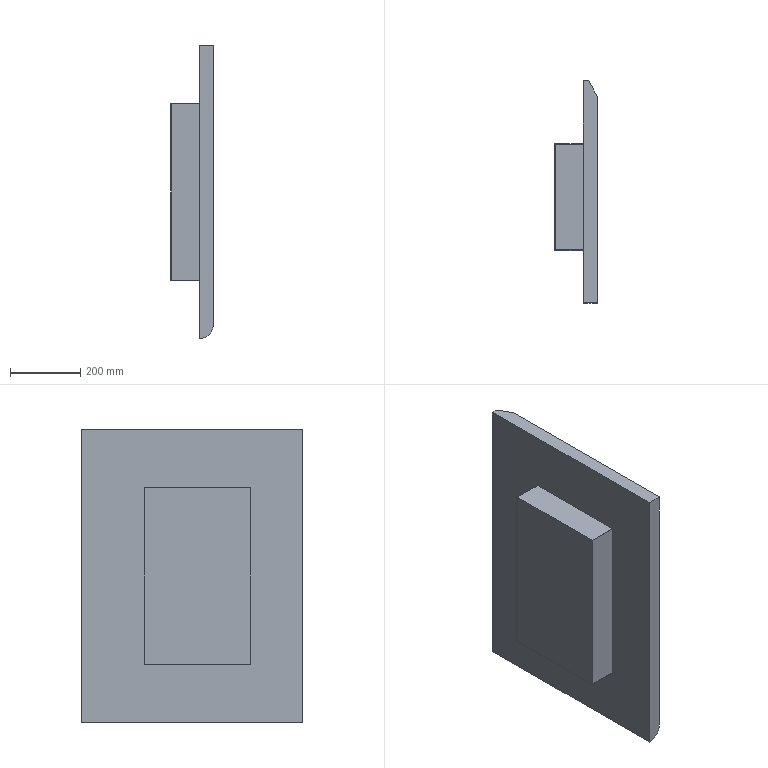Part | SolidWorks | features ICE 2, BossThin 1, CutThin 1, Extrusion 1, Fillet 1 | 1 solid | 27 faces | box 121.2 x 630 x 832.5 mm | volume 14657432 mm3 | plane 26 | cylinder 1 | commonest cylinder face diameters 80 x1
STEP:
#1=CARTESIAN_POINT('',(15.,0.,832.5));
#2=VERTEX_POINT('',#1);
#3=CARTESIAN_POINT('',(15.,0.,2.919));
#4=VERTEX_POINT('',#3);
#5=CARTESIAN_POINT('',(15.,0.,832.5));
#6=DIRECTION('',(0.,0.,-1.));
#7=VECTOR('',#6,1000.);
#8=LINE('',#5,#7);
#9=EDGE_CURVE('',#2,#4,#8,.T.);
#10=ORIENTED_EDGE('',*,*,#9,.T.);
#11=CARTESIAN_POINT('',(0.,0.,0.));
#12=VERTEX_POINT('',#11);
#13=CARTESIAN_POINT('',(0.,0.,40.));
#14=DIRECTION('',(0.,1.,0.));
#15=DIRECTION('',(0.,0.,-1.));
#16=AXIS2_PLACEMENT_3D('',#13,#14,#15);
#17=CIRCLE('',#16,40.);
#18=EDGE_CURVE('',#4,#12,#17,.T.);
#19=ORIENTED_EDGE('',*,*,#18,.T.);
#20=CARTESIAN_POINT('',(0.,0.,832.5));
#21=VERTEX_POINT('',#20);
#22=CARTESIAN_POINT('',(0.,0.,832.5));
#23=DIRECTION('',(0.,0.,-1.));
#24=VECTOR('',#23,1000.);
#25=LINE('',#22,#24);
#26=EDGE_CURVE('',#21,#12,#25,.T.);
#27=ORIENTED_EDGE('',*,*,#26,.F.);
#28=CARTESIAN_POINT('',(0.,0.,832.5));
#29=DIRECTION('',(-1.,0.,0.));
#30=VECTOR('',#29,1000.);
#31=LINE('',#28,#30);
#32=EDGE_CURVE('',#2,#21,#31,.T.);
#33=ORIENTED_EDGE('',*,*,#32,.F.);
#34=EDGE_LOOP('',(#10,#19,#27,#33));
#35=FACE_OUTER_BOUND('',#34,.T.);
#36=CARTESIAN_POINT('',(0.,0.,832.5));
#37=DIRECTION('',(0.,-1.,0.));
#38=DIRECTION('',(0.,0.,-1.));
#39=AXIS2_PLACEMENT_3D('',#36,#37,#38);
#40=PLANE('',#39);
#41=ADVANCED_FACE('',(#35),#40,.F.);
#42=CARTESIAN_POINT('',(0.,-178.8,165.05));
#43=VERTEX_POINT('',#42);
#44=CARTESIAN_POINT('',(0.,-178.8,667.45));
#45=VERTEX_POINT('',#44);
#46=CARTESIAN_POINT('',(0.,-178.8,832.5));
#47=DIRECTION('',(0.,0.,1.));
#48=VECTOR('',#47,1000.);
#49=LINE('',#46,#48);
#50=EDGE_CURVE('',#43,#45,#49,.T.);
#51=ORIENTED_EDGE('',*,*,#50,.T.);
#52=CARTESIAN_POINT('',(0.,-481.2,667.45));
#53=VERTEX_POINT('',#52);
#54=CARTESIAN_POINT('',(0.,0.,667.45));
#55=DIRECTION('',(0.,-1.,0.));
#56=VECTOR('',#55,1000.);
#57=LINE('',#54,#56);
#58=EDGE_CURVE('',#45,#53,#57,.T.);
#59=ORIENTED_EDGE('',*,*,#58,.T.);
#60=CARTESIAN_POINT('',(0.,-481.2,165.05));
#61=VERTEX_POINT('',#60);
#62=CARTESIAN_POINT('',(0.,-481.2,832.5));
#63=DIRECTION('',(0.,0.,-1.));
#64=VECTOR('',#63,1000.);
#65=LINE('',#62,#64);
#66=EDGE_CURVE('',#53,#61,#65,.T.);
#67=ORIENTED_EDGE('',*,*,#66,.T.);
#68=CARTESIAN_POINT('',(0.,0.,165.05));
#69=DIRECTION('',(0.,1.,0.));
#70=VECTOR('',#69,1000.);
#71=LINE('',#68,#70);
#72=EDGE_CURVE('',#61,#43,#71,.T.);
#73=ORIENTED_EDGE('',*,*,#72,.T.);
#74=EDGE_LOOP('',(#51,#59,#67,#73));
#75=FACE_BOUND('',#74,.T.);
#76=CARTESIAN_POINT('',(0.,-630.,0.));
#77=VERTEX_POINT('',#76);
#78=CARTESIAN_POINT('',(0.,0.,0.));
#79=DIRECTION('',(0.,-1.,0.));
#80=VECTOR('',#79,1000.);
#81=LINE('',#78,#80);
#82=EDGE_CURVE('',#12,#77,#81,.T.);
#83=ORIENTED_EDGE('',*,*,#82,.T.);
#84=CARTESIAN_POINT('',(0.,-630.,832.5));
#85=VERTEX_POINT('',#84);
#86=CARTESIAN_POINT('',(0.,-630.,832.5));
#87=DIRECTION('',(0.,0.,-1.));
#88=VECTOR('',#87,1000.);
#89=LINE('',#86,#88);
#90=EDGE_CURVE('',#85,#77,#89,.T.);
#91=ORIENTED_EDGE('',*,*,#90,.F.);
#92=CARTESIAN_POINT('',(0.,0.,832.5));
#93=DIRECTION('',(0.,-1.,0.));
#94=VECTOR('',#93,1000.);
#95=LINE('',#92,#94);
#96=EDGE_CURVE('',#21,#85,#95,.T.);
#97=ORIENTED_EDGE('',*,*,#96,.F.);
#98=ORIENTED_EDGE('',*,*,#26,.T.);
#99=EDGE_LOOP('',(#83,#91,#97,#98));
#100=FACE_OUTER_BOUND('',#99,.T.);
#101=CARTESIAN_POINT('',(0.,0.,832.5));
#102=DIRECTION('',(1.,0.,0.));
#103=DIRECTION('',(0.,1.,0.));
#104=AXIS2_PLACEMENT_3D('',#101,#102,#103);
#105=PLANE('',#104);
#106=ADVANCED_FACE('',(#75,#100),#105,.F.);
#107=ORIENTED_EDGE('',*,*,#90,.T.);
#108=CARTESIAN_POINT('',(40.,-630.,40.));
#109=VERTEX_POINT('',#108);
#110=CARTESIAN_POINT('',(0.,-630.,40.));
#111=DIRECTION('',(0.,-1.,0.));
#112=DIRECTION('',(0.,0.,1.));
#113=AXIS2_PLACEMENT_3D('',#110,#111,#112);
#114=CIRCLE('',#113,40.);
#115=EDGE_CURVE('',#77,#109,#114,.T.);
#116=ORIENTED_EDGE('',*,*,#115,.T.);
#117=CARTESIAN_POINT('',(40.,-630.,832.5));
#118=VERTEX_POINT('',#117);
#119=CARTESIAN_POINT('',(40.,-630.,832.5));
#120=DIRECTION('',(0.,0.,-1.));
#121=VECTOR('',#120,1000.);
#122=LINE('',#119,#121);
#123=EDGE_CURVE('',#118,#109,#122,.T.);
#124=ORIENTED_EDGE('',*,*,#123,.F.);
#125=CARTESIAN_POINT('',(0.,-630.,832.5));
#126=DIRECTION('',(1.,0.,0.));
#127=VECTOR('',#126,1000.);
#128=LINE('',#125,#127);
#129=EDGE_CURVE('',#85,#118,#128,.T.);
#130=ORIENTED_EDGE('',*,*,#129,.F.);
#131=EDGE_LOOP('',(#107,#116,#124,#130));
#132=FACE_OUTER_BOUND('',#131,.T.);
#133=CARTESIAN_POINT('',(0.,-630.,832.5));
#134=DIRECTION('',(0.,1.,0.));
#135=DIRECTION('',(0.,0.,1.));
#136=AXIS2_PLACEMENT_3D('',#133,#134,#135);
#137=PLANE('',#136);
#138=ADVANCED_FACE('',(#132),#137,.F.);
#139=CARTESIAN_POINT('',(40.,-144.501,465.45));
#140=VERTEX_POINT('',#139);
#141=CARTESIAN_POINT('',(40.,-144.501,367.05));
#142=VERTEX_POINT('',#141);
#143=CARTESIAN_POINT('',(40.,-144.501,464.25));
#144=DIRECTION('',(0.,0.,-1.));
#145=VECTOR('',#144,1000.);
#146=LINE('',#143,#145);
#147=EDGE_CURVE('',#140,#142,#146,.T.);
#148=ORIENTED_EDGE('',*,*,#147,.F.);
#149=CARTESIAN_POINT('',(40.,-102.101,465.45));
#150=VERTEX_POINT('',#149);
#151=CARTESIAN_POINT('',(40.,-103.301,465.45));
#152=DIRECTION('',(0.,-1.,0.));
#153=VECTOR('',#152,1000.);
#154=LINE('',#151,#153);
#155=EDGE_CURVE('',#150,#140,#154,.T.);
#156=ORIENTED_EDGE('',*,*,#155,.F.);
#157=CARTESIAN_POINT('',(40.,-102.101,367.05));
#158=VERTEX_POINT('',#157);
#159=CARTESIAN_POINT('',(40.,-102.101,464.25));
#160=DIRECTION('',(0.,0.,1.));
#161=VECTOR('',#160,1000.);
#162=LINE('',#159,#161);
#163=EDGE_CURVE('',#158,#150,#162,.T.);
#164=ORIENTED_EDGE('',*,*,#163,.F.);
#165=CARTESIAN_POINT('',(40.,-103.301,367.05));
#166=DIRECTION('',(0.,1.,0.));
#167=VECTOR('',#166,1000.);
#168=LINE('',#165,#167);
#169=EDGE_CURVE('',#142,#158,#168,.T.);
#170=ORIENTED_EDGE('',*,*,#169,.F.);
#171=EDGE_LOOP('',(#148,#156,#164,#170));
#172=FACE_BOUND('',#171,.T.);
#173=ORIENTED_EDGE('',*,*,#123,.T.);
#174=CARTESIAN_POINT('',(40.,-43.301,40.));
#175=VERTEX_POINT('',#174);
#176=CARTESIAN_POINT('',(40.,-630.,40.));
#177=DIRECTION('',(0.,1.,0.));
#178=VECTOR('',#177,1000.);
#179=LINE('',#176,#178);
#180=EDGE_CURVE('',#109,#175,#179,.T.);
#181=ORIENTED_EDGE('',*,*,#180,.T.);
#182=CARTESIAN_POINT('',(40.,-43.301,832.5));
#183=VERTEX_POINT('',#182);
#184=CARTESIAN_POINT('',(40.,-43.301,832.5));
#185=DIRECTION('',(0.,0.,-1.));
#186=VECTOR('',#185,1000.);
#187=LINE('',#184,#186);
#188=EDGE_CURVE('',#183,#175,#187,.T.);
#189=ORIENTED_EDGE('',*,*,#188,.F.);
#190=CARTESIAN_POINT('',(40.,-630.,832.5));
#191=DIRECTION('',(0.,1.,0.));
#192=VECTOR('',#191,1000.);
#193=LINE('',#190,#192);
#194=EDGE_CURVE('',#118,#183,#193,.T.);
#195=ORIENTED_EDGE('',*,*,#194,.F.);
#196=EDGE_LOOP('',(#173,#181,#189,#195));
#197=FACE_OUTER_BOUND('',#196,.T.);
#198=CARTESIAN_POINT('',(40.,-480.,666.25));
#199=VERTEX_POINT('',#198);
#200=CARTESIAN_POINT('',(40.,-480.,166.25));
#201=VERTEX_POINT('',#200);
#202=CARTESIAN_POINT('',(40.,-480.,666.25));
#203=DIRECTION('',(0.,0.,-1.));
#204=VECTOR('',#203,1000.);
#205=LINE('',#202,#204);
#206=EDGE_CURVE('',#199,#201,#205,.T.);
#207=ORIENTED_EDGE('',*,*,#206,.F.);
#208=CARTESIAN_POINT('',(40.,-180.,666.25));
#209=VERTEX_POINT('',#208);
#210=CARTESIAN_POINT('',(40.,-180.,666.25));
#211=DIRECTION('',(0.,-1.,0.));
#212=VECTOR('',#211,1000.);
#213=LINE('',#210,#212);
#214=EDGE_CURVE('',#209,#199,#213,.T.);
#215=ORIENTED_EDGE('',*,*,#214,.F.);
#216=CARTESIAN_POINT('',(40.,-180.,166.25));
#217=VERTEX_POINT('',#216);
#218=CARTESIAN_POINT('',(40.,-180.,666.25));
#219=DIRECTION('',(0.,0.,1.));
#220=VECTOR('',#219,1000.);
#221=LINE('',#218,#220);
#222=EDGE_CURVE('',#217,#209,#221,.T.);
#223=ORIENTED_EDGE('',*,*,#222,.F.);
#224=CARTESIAN_POINT('',(40.,-180.,166.25));
#225=DIRECTION('',(0.,1.,0.));
#226=VECTOR('',#225,1000.);
#227=LINE('',#224,#226);
#228=EDGE_CURVE('',#201,#217,#227,.T.);
#229=ORIENTED_EDGE('',*,*,#228,.F.);
#230=EDGE_LOOP('',(#207,#215,#223,#229));
#231=FACE_BOUND('',#230,.T.);
#232=CARTESIAN_POINT('',(40.,-630.,832.5));
#233=DIRECTION('',(-1.,0.,0.));
#234=DIRECTION('',(0.,-1.,0.));
#235=AXIS2_PLACEMENT_3D('',#232,#233,#234);
#236=PLANE('',#235);
#237=ADVANCED_FACE('',(#172,#197,#231),#236,.F.);
#238=ORIENTED_EDGE('',*,*,#188,.T.);
#239=CARTESIAN_POINT('',(40.,-43.301,40.));
#240=CARTESIAN_POINT('',(40.,-43.301,23.177));
#241=CARTESIAN_POINT('',(30.596,-27.012,9.228));
#242=CARTESIAN_POINT('',(15.,0.,2.919));
#243=(BOUNDED_CURVE()B_SPLINE_CURVE(3,(#239,#240,#241,#242),.UNSPECIFIED.,.F.,.F.)B_SPLINE_CURVE_WITH_KNOTS((4,4),(3.142,4.328),.UNSPECIFIED.)CURVE()GEOMETRIC_REPRESENTATION_ITEM()RATIONAL_B_SPLINE_CURVE((1.,0.8861,0.8861,1.))REPRESENTATION_ITEM(''));
#244=EDGE_CURVE('',#175,#4,#243,.T.);
#245=ORIENTED_EDGE('',*,*,#244,.T.);
#246=ORIENTED_EDGE('',*,*,#9,.F.);
#247=CARTESIAN_POINT('',(15.,0.,832.5));
#248=DIRECTION('',(-0.5,0.866,0.));
#249=VECTOR('',#248,1000.);
#250=LINE('',#247,#249);
#251=EDGE_CURVE('',#183,#2,#250,.T.);
#252=ORIENTED_EDGE('',*,*,#251,.F.);
#253=EDGE_LOOP('',(#238,#245,#246,#252));
#254=FACE_OUTER_BOUND('',#253,.T.);
#255=CARTESIAN_POINT('',(15.,0.,832.5));
#256=DIRECTION('',(-0.866,-0.5,0.));
#257=DIRECTION('',(0.5,-0.866,0.));
#258=AXIS2_PLACEMENT_3D('',#255,#256,#257);
#259=PLANE('',#258);
#260=ADVANCED_FACE('',(#254),#259,.F.);
#261=ORIENTED_EDGE('',*,*,#32,.T.);
#262=ORIENTED_EDGE('',*,*,#96,.T.);
#263=ORIENTED_EDGE('',*,*,#129,.T.);
#264=ORIENTED_EDGE('',*,*,#194,.T.);
#265=ORIENTED_EDGE('',*,*,#251,.T.);
#266=EDGE_LOOP('',(#261,#262,#263,#264,#265));
#267=FACE_OUTER_BOUND('',#266,.T.);
#268=CARTESIAN_POINT('',(0.,0.,832.5));
#269=DIRECTION('',(0.,0.,1.));
#270=DIRECTION('',(1.,0.,0.));
#271=AXIS2_PLACEMENT_3D('',#268,#269,#270);
#272=PLANE('',#271);
#273=ADVANCED_FACE('',(#267),#272,.T.);
#274=ORIENTED_EDGE('',*,*,#155,.T.);
#275=CARTESIAN_POINT('',(38.,-144.501,465.45));
#276=VERTEX_POINT('',#275);
#277=CARTESIAN_POINT('',(38.,-144.501,465.45));
#278=DIRECTION('',(1.,0.,0.));
#279=VECTOR('',#278,1000.);
#280=LINE('',#277,#279);
#281=EDGE_CURVE('',#276,#140,#280,.T.);
#282=ORIENTED_EDGE('',*,*,#281,.F.);
#283=CARTESIAN_POINT('',(38.,-102.101,465.45));
#284=VERTEX_POINT('',#283);
#285=CARTESIAN_POINT('',(38.,-103.301,465.45));
#286=DIRECTION('',(0.,-1.,0.));
#287=VECTOR('',#286,1000.);
#288=LINE('',#285,#287);
#289=EDGE_CURVE('',#284,#276,#288,.T.);
#290=ORIENTED_EDGE('',*,*,#289,.F.);
#291=CARTESIAN_POINT('',(38.,-102.101,465.45));
#292=DIRECTION('',(1.,0.,0.));
#293=VECTOR('',#292,1000.);
#294=LINE('',#291,#293);
#295=EDGE_CURVE('',#284,#150,#294,.T.);
#296=ORIENTED_EDGE('',*,*,#295,.T.);
#297=EDGE_LOOP('',(#274,#282,#290,#296));
#298=FACE_OUTER_BOUND('',#297,.T.);
#299=CARTESIAN_POINT('',(38.,-103.301,465.45));
#300=DIRECTION('',(0.,0.,1.));
#301=DIRECTION('',(1.,0.,0.));
#302=AXIS2_PLACEMENT_3D('',#299,#300,#301);
#303=PLANE('',#302);
#304=ADVANCED_FACE('',(#298),#303,.F.);
#305=ORIENTED_EDGE('',*,*,#163,.T.);
#306=ORIENTED_EDGE('',*,*,#295,.F.);
#307=CARTESIAN_POINT('',(38.,-102.101,367.05));
#308=VERTEX_POINT('',#307);
#309=CARTESIAN_POINT('',(38.,-102.101,464.25));
#310=DIRECTION('',(0.,0.,1.));
#311=VECTOR('',#310,1000.);
#312=LINE('',#309,#311);
#313=EDGE_CURVE('',#308,#284,#312,.T.);
#314=ORIENTED_EDGE('',*,*,#313,.F.);
#315=CARTESIAN_POINT('',(38.,-102.101,367.05));
#316=DIRECTION('',(1.,0.,0.));
#317=VECTOR('',#316,1000.);
#318=LINE('',#315,#317);
#319=EDGE_CURVE('',#308,#158,#318,.T.);
#320=ORIENTED_EDGE('',*,*,#319,.T.);
#321=EDGE_LOOP('',(#305,#306,#314,#320));
#322=FACE_OUTER_BOUND('',#321,.T.);
#323=CARTESIAN_POINT('',(38.,-102.101,464.25));
#324=DIRECTION('',(0.,1.,0.));
#325=DIRECTION('',(0.,0.,1.));
#326=AXIS2_PLACEMENT_3D('',#323,#324,#325);
#327=PLANE('',#326);
#328=ADVANCED_FACE('',(#322),#327,.F.);
#329=ORIENTED_EDGE('',*,*,#169,.T.);
#330=ORIENTED_EDGE('',*,*,#319,.F.);
#331=CARTESIAN_POINT('',(38.,-144.501,367.05));
#332=VERTEX_POINT('',#331);
#333=CARTESIAN_POINT('',(38.,-103.301,367.05));
#334=DIRECTION('',(0.,1.,0.));
#335=VECTOR('',#334,1000.);
#336=LINE('',#333,#335);
#337=EDGE_CURVE('',#332,#308,#336,.T.);
#338=ORIENTED_EDGE('',*,*,#337,.F.);
#339=CARTESIAN_POINT('',(38.,-144.501,367.05));
#340=DIRECTION('',(1.,0.,0.));
#341=VECTOR('',#340,1000.);
#342=LINE('',#339,#341);
#343=EDGE_CURVE('',#332,#142,#342,.T.);
#344=ORIENTED_EDGE('',*,*,#343,.T.);
#345=EDGE_LOOP('',(#329,#330,#338,#344));
#346=FACE_OUTER_BOUND('',#345,.T.);
#347=CARTESIAN_POINT('',(38.,-103.301,367.05));
#348=DIRECTION('',(0.,0.,-1.));
#349=DIRECTION('',(0.,1.,0.));
#350=AXIS2_PLACEMENT_3D('',#347,#348,#349);
#351=PLANE('',#350);
#352=ADVANCED_FACE('',(#346),#351,.F.);
#353=ORIENTED_EDGE('',*,*,#147,.T.);
#354=ORIENTED_EDGE('',*,*,#343,.F.);
#355=CARTESIAN_POINT('',(38.,-144.501,464.25));
#356=DIRECTION('',(0.,0.,-1.));
#357=VECTOR('',#356,1000.);
#358=LINE('',#355,#357);
#359=EDGE_CURVE('',#276,#332,#358,.T.);
#360=ORIENTED_EDGE('',*,*,#359,.F.);
#361=ORIENTED_EDGE('',*,*,#281,.T.);
#362=EDGE_LOOP('',(#353,#354,#360,#361));
#363=FACE_OUTER_BOUND('',#362,.T.);
#364=CARTESIAN_POINT('',(38.,-144.501,464.25));
#365=DIRECTION('',(0.,-1.,0.));
#366=DIRECTION('',(1.,0.,0.));
#367=AXIS2_PLACEMENT_3D('',#364,#365,#366);
#368=PLANE('',#367);
#369=ADVANCED_FACE('',(#363),#368,.F.);
#370=CARTESIAN_POINT('',(38.,-103.301,368.25));
#371=VERTEX_POINT('',#370);
#372=CARTESIAN_POINT('',(38.,-103.301,464.25));
#373=VERTEX_POINT('',#372);
#374=CARTESIAN_POINT('',(38.,-103.301,464.25));
#375=DIRECTION('',(0.,0.,1.));
#376=VECTOR('',#375,1000.);
#377=LINE('',#374,#376);
#378=EDGE_CURVE('',#371,#373,#377,.T.);
#379=ORIENTED_EDGE('',*,*,#378,.F.);
#380=CARTESIAN_POINT('',(38.,-143.301,368.25));
#381=VERTEX_POINT('',#380);
#382=CARTESIAN_POINT('',(38.,-103.301,368.25));
#383=DIRECTION('',(0.,1.,0.));
#384=VECTOR('',#383,1000.);
#385=LINE('',#382,#384);
#386=EDGE_CURVE('',#381,#371,#385,.T.);
#387=ORIENTED_EDGE('',*,*,#386,.F.);
#388=CARTESIAN_POINT('',(38.,-143.301,464.25));
#389=VERTEX_POINT('',#388);
#390=CARTESIAN_POINT('',(38.,-143.301,464.25));
#391=DIRECTION('',(0.,0.,-1.));
#392=VECTOR('',#391,1000.);
#393=LINE('',#390,#392);
#394=EDGE_CURVE('',#389,#381,#393,.T.);
#395=ORIENTED_EDGE('',*,*,#394,.F.);
#396=CARTESIAN_POINT('',(38.,-103.301,464.25));
#397=DIRECTION('',(0.,-1.,0.));
#398=VECTOR('',#397,1000.);
#399=LINE('',#396,#398);
#400=EDGE_CURVE('',#373,#389,#399,.T.);
#401=ORIENTED_EDGE('',*,*,#400,.F.);
#402=EDGE_LOOP('',(#379,#387,#395,#401));
#403=FACE_BOUND('',#402,.T.);
#404=ORIENTED_EDGE('',*,*,#289,.T.);
#405=ORIENTED_EDGE('',*,*,#359,.T.);
#406=ORIENTED_EDGE('',*,*,#337,.T.);
#407=ORIENTED_EDGE('',*,*,#313,.T.);
#408=EDGE_LOOP('',(#404,#405,#406,#407));
#409=FACE_OUTER_BOUND('',#408,.T.);
#410=CARTESIAN_POINT('',(38.,0.,0.));
#411=DIRECTION('',(1.,0.,0.));
#412=DIRECTION('',(0.,0.,-1.));
#413=AXIS2_PLACEMENT_3D('',#410,#411,#412);
#414=PLANE('',#413);
#415=ADVANCED_FACE('',(#403,#409),#414,.T.);
#416=CARTESIAN_POINT('',(40.,-103.301,464.25));
#417=VERTEX_POINT('',#416);
#418=CARTESIAN_POINT('',(40.,-143.301,464.25));
#419=VERTEX_POINT('',#418);
#420=CARTESIAN_POINT('',(40.,-103.301,464.25));
#421=DIRECTION('',(0.,-1.,0.));
#422=VECTOR('',#421,1000.);
#423=LINE('',#420,#422);
#424=EDGE_CURVE('',#417,#419,#423,.T.);
#425=ORIENTED_EDGE('',*,*,#424,.F.);
#426=CARTESIAN_POINT('',(38.,-103.301,464.25));
#427=DIRECTION('',(1.,0.,0.));
#428=VECTOR('',#427,1000.);
#429=LINE('',#426,#428);
#430=EDGE_CURVE('',#373,#417,#429,.T.);
#431=ORIENTED_EDGE('',*,*,#430,.F.);
#432=ORIENTED_EDGE('',*,*,#400,.T.);
#433=CARTESIAN_POINT('',(38.,-143.301,464.25));
#434=DIRECTION('',(1.,0.,0.));
#435=VECTOR('',#434,1000.);
#436=LINE('',#433,#435);
#437=EDGE_CURVE('',#389,#419,#436,.T.);
#438=ORIENTED_EDGE('',*,*,#437,.T.);
#439=EDGE_LOOP('',(#425,#431,#432,#438));
#440=FACE_OUTER_BOUND('',#439,.T.);
#441=CARTESIAN_POINT('',(38.,-103.301,464.25));
#442=DIRECTION('',(0.,0.,1.));
#443=DIRECTION('',(1.,0.,0.));
#444=AXIS2_PLACEMENT_3D('',#441,#442,#443);
#445=PLANE('',#444);
#446=ADVANCED_FACE('',(#440),#445,.T.);
#447=CARTESIAN_POINT('',(40.,-103.301,368.25));
#448=VERTEX_POINT('',#447);
#449=CARTESIAN_POINT('',(40.,-103.301,464.25));
#450=DIRECTION('',(0.,0.,1.));
#451=VECTOR('',#450,1000.);
#452=LINE('',#449,#451);
#453=EDGE_CURVE('',#448,#417,#452,.T.);
#454=ORIENTED_EDGE('',*,*,#453,.F.);
#455=CARTESIAN_POINT('',(38.,-103.301,368.25));
#456=DIRECTION('',(1.,0.,0.));
#457=VECTOR('',#456,1000.);
#458=LINE('',#455,#457);
#459=EDGE_CURVE('',#371,#448,#458,.T.);
#460=ORIENTED_EDGE('',*,*,#459,.F.);
#461=ORIENTED_EDGE('',*,*,#378,.T.);
#462=ORIENTED_EDGE('',*,*,#430,.T.);
#463=EDGE_LOOP('',(#454,#460,#461,#462));
#464=FACE_OUTER_BOUND('',#463,.T.);
#465=CARTESIAN_POINT('',(38.,-103.301,464.25));
#466=DIRECTION('',(0.,1.,0.));
#467=DIRECTION('',(0.,0.,1.));
#468=AXIS2_PLACEMENT_3D('',#465,#466,#467);
#469=PLANE('',#468);
#470=ADVANCED_FACE('',(#464),#469,.T.);
#471=CARTESIAN_POINT('',(40.,-143.301,368.25));
#472=VERTEX_POINT('',#471);
#473=CARTESIAN_POINT('',(40.,-103.301,368.25));
#474=DIRECTION('',(0.,1.,0.));
#475=VECTOR('',#474,1000.);
#476=LINE('',#473,#475);
#477=EDGE_CURVE('',#472,#448,#476,.T.);
#478=ORIENTED_EDGE('',*,*,#477,.F.);
#479=CARTESIAN_POINT('',(38.,-143.301,368.25));
#480=DIRECTION('',(1.,0.,0.));
#481=VECTOR('',#480,1000.);
#482=LINE('',#479,#481);
#483=EDGE_CURVE('',#381,#472,#482,.T.);
#484=ORIENTED_EDGE('',*,*,#483,.F.);
#485=ORIENTED_EDGE('',*,*,#386,.T.);
#486=ORIENTED_EDGE('',*,*,#459,.T.);
#487=EDGE_LOOP('',(#478,#484,#485,#486));
#488=FACE_OUTER_BOUND('',#487,.T.);
#489=CARTESIAN_POINT('',(38.,-103.301,368.25));
#490=DIRECTION('',(0.,0.,-1.));
#491=DIRECTION('',(0.,1.,0.));
#492=AXIS2_PLACEMENT_3D('',#489,#490,#491);
#493=PLANE('',#492);
#494=ADVANCED_FACE('',(#488),#493,.T.);
#495=CARTESIAN_POINT('',(40.,-143.301,464.25));
#496=DIRECTION('',(0.,0.,-1.));
#497=VECTOR('',#496,1000.);
#498=LINE('',#495,#497);
#499=EDGE_CURVE('',#419,#472,#498,.T.);
#500=ORIENTED_EDGE('',*,*,#499,.F.);
#501=ORIENTED_EDGE('',*,*,#437,.F.);
#502=ORIENTED_EDGE('',*,*,#394,.T.);
#503=ORIENTED_EDGE('',*,*,#483,.T.);
#504=EDGE_LOOP('',(#500,#501,#502,#503));
#505=FACE_OUTER_BOUND('',#504,.T.);
#506=CARTESIAN_POINT('',(38.,-143.301,464.25));
#507=DIRECTION('',(0.,-1.,0.));
#508=DIRECTION('',(1.,0.,0.));
#509=AXIS2_PLACEMENT_3D('',#506,#507,#508);
#510=PLANE('',#509);
#511=ADVANCED_FACE('',(#505),#510,.T.);
#512=ORIENTED_EDGE('',*,*,#424,.T.);
#513=ORIENTED_EDGE('',*,*,#499,.T.);
#514=ORIENTED_EDGE('',*,*,#477,.T.);
#515=ORIENTED_EDGE('',*,*,#453,.T.);
#516=EDGE_LOOP('',(#512,#513,#514,#515));
#517=FACE_OUTER_BOUND('',#516,.T.);
#518=CARTESIAN_POINT('',(40.,-630.,832.5));
#519=DIRECTION('',(-1.,0.,0.));
#520=DIRECTION('',(0.,-1.,0.));
#521=AXIS2_PLACEMENT_3D('',#518,#519,#520);
#522=PLANE('',#521);
#523=ADVANCED_FACE('',(#517),#522,.F.);
#524=ORIENTED_EDGE('',*,*,#115,.F.);
#525=ORIENTED_EDGE('',*,*,#82,.F.);
#526=ORIENTED_EDGE('',*,*,#18,.F.);
#527=ORIENTED_EDGE('',*,*,#244,.F.);
#528=ORIENTED_EDGE('',*,*,#180,.F.);
#529=EDGE_LOOP('',(#524,#525,#526,#527,#528));
#530=FACE_OUTER_BOUND('',#529,.T.);
#531=CARTESIAN_POINT('',(0.,-630.,40.));
#532=DIRECTION('',(0.,1.,0.));
#533=DIRECTION('',(-1.,0.,0.));
#534=AXIS2_PLACEMENT_3D('',#531,#532,#533);
#535=CYLINDRICAL_SURFACE('',#534,40.);
#536=ADVANCED_FACE('',(#530),#535,.T.);
#537=ORIENTED_EDGE('',*,*,#214,.T.);
#538=CARTESIAN_POINT('',(-80.,-480.,666.25));
#539=VERTEX_POINT('',#538);
#540=CARTESIAN_POINT('',(0.,-480.,666.25));
#541=DIRECTION('',(1.,0.,0.));
#542=VECTOR('',#541,1000.);
#543=LINE('',#540,#542);
#544=EDGE_CURVE('',#539,#199,#543,.T.);
#545=ORIENTED_EDGE('',*,*,#544,.F.);
#546=CARTESIAN_POINT('',(-80.,-180.,666.25));
#547=VERTEX_POINT('',#546);
#548=CARTESIAN_POINT('',(-80.,-180.,666.25));
#549=DIRECTION('',(0.,-1.,0.));
#550=VECTOR('',#549,1000.);
#551=LINE('',#548,#550);
#552=EDGE_CURVE('',#547,#539,#551,.T.);
#553=ORIENTED_EDGE('',*,*,#552,.F.);
#554=CARTESIAN_POINT('',(0.,-180.,666.25));
#555=DIRECTION('',(1.,0.,0.));
#556=VECTOR('',#555,1000.);
#557=LINE('',#554,#556);
#558=EDGE_CURVE('',#547,#209,#557,.T.);
#559=ORIENTED_EDGE('',*,*,#558,.T.);
#560=EDGE_LOOP('',(#537,#545,#553,#559));
#561=FACE_OUTER_BOUND('',#560,.T.);
#562=CARTESIAN_POINT('',(0.,-180.,666.25));
#563=DIRECTION('',(0.,0.,1.));
#564=DIRECTION('',(0.,-1.,0.));
#565=AXIS2_PLACEMENT_3D('',#562,#563,#564);
#566=PLANE('',#565);
#567=ADVANCED_FACE('',(#561),#566,.F.);
#568=ORIENTED_EDGE('',*,*,#222,.T.);
#569=ORIENTED_EDGE('',*,*,#558,.F.);
#570=CARTESIAN_POINT('',(-80.,-180.,166.25));
#571=VERTEX_POINT('',#570);
#572=CARTESIAN_POINT('',(-80.,-180.,166.25));
#573=DIRECTION('',(0.,0.,1.));
#574=VECTOR('',#573,1000.);
#575=LINE('',#572,#574);
#576=EDGE_CURVE('',#571,#547,#575,.T.);
#577=ORIENTED_EDGE('',*,*,#576,.F.);
#578=CARTESIAN_POINT('',(0.,-180.,166.25));
#579=DIRECTION('',(1.,0.,0.));
#580=VECTOR('',#579,1000.);
#581=LINE('',#578,#580);
#582=EDGE_CURVE('',#571,#217,#581,.T.);
#583=ORIENTED_EDGE('',*,*,#582,.T.);
#584=EDGE_LOOP('',(#568,#569,#577,#583));
#585=FACE_OUTER_BOUND('',#584,.T.);
#586=CARTESIAN_POINT('',(0.,-180.,666.25));
#587=DIRECTION('',(0.,1.,0.));
#588=DIRECTION('',(0.,0.,1.));
#589=AXIS2_PLACEMENT_3D('',#586,#587,#588);
#590=PLANE('',#589);
#591=ADVANCED_FACE('',(#585),#590,.F.);
#592=ORIENTED_EDGE('',*,*,#228,.T.);
#593=ORIENTED_EDGE('',*,*,#582,.F.);
#594=CARTESIAN_POINT('',(-80.,-480.,166.25));
#595=VERTEX_POINT('',#594);
#596=CARTESIAN_POINT('',(-80.,-480.,166.25));
#597=DIRECTION('',(0.,1.,0.));
#598=VECTOR('',#597,1000.);
#599=LINE('',#596,#598);
#600=EDGE_CURVE('',#595,#571,#599,.T.);
#601=ORIENTED_EDGE('',*,*,#600,.F.);
#602=CARTESIAN_POINT('',(0.,-480.,166.25));
#603=DIRECTION('',(1.,0.,0.));
#604=VECTOR('',#603,1000.);
#605=LINE('',#602,#604);
#606=EDGE_CURVE('',#595,#201,#605,.T.);
#607=ORIENTED_EDGE('',*,*,#606,.T.);
#608=EDGE_LOOP('',(#592,#593,#601,#607));
#609=FACE_OUTER_BOUND('',#608,.T.);
#610=CARTESIAN_POINT('',(0.,-180.,166.25));
#611=DIRECTION('',(0.,0.,-1.));
#612=DIRECTION('',(-1.,0.,0.));
#613=AXIS2_PLACEMENT_3D('',#610,#611,#612);
#614=PLANE('',#613);
#615=ADVANCED_FACE('',(#609),#614,.F.);
#616=ORIENTED_EDGE('',*,*,#206,.T.);
#617=ORIENTED_EDGE('',*,*,#606,.F.);
#618=CARTESIAN_POINT('',(-80.,-480.,666.25));
#619=DIRECTION('',(0.,0.,-1.));
#620=VECTOR('',#619,1000.);
#621=LINE('',#618,#620);
#622=EDGE_CURVE('',#539,#595,#621,.T.);
#623=ORIENTED_EDGE('',*,*,#622,.F.);
#624=ORIENTED_EDGE('',*,*,#544,.T.);
#625=EDGE_LOOP('',(#616,#617,#623,#624));
#626=FACE_OUTER_BOUND('',#625,.T.);
#627=CARTESIAN_POINT('',(0.,-480.,666.25));
#628=DIRECTION('',(0.,-1.,0.));
#629=DIRECTION('',(0.,0.,-1.));
#630=AXIS2_PLACEMENT_3D('',#627,#628,#629);
#631=PLANE('',#630);
#632=ADVANCED_FACE('',(#626),#631,.F.);
#633=ORIENTED_EDGE('',*,*,#58,.F.);
#634=CARTESIAN_POINT('',(-81.2,-178.8,667.45));
#635=VERTEX_POINT('',#634);
#636=CARTESIAN_POINT('',(-80.,-178.8,667.45));
#637=DIRECTION('',(1.,0.,0.));
#638=VECTOR('',#637,1000.);
#639=LINE('',#636,#638);
#640=EDGE_CURVE('',#635,#45,#639,.T.);
#641=ORIENTED_EDGE('',*,*,#640,.F.);
#642=CARTESIAN_POINT('',(-81.2,-481.2,667.45));
#643=VERTEX_POINT('',#642);
#644=CARTESIAN_POINT('',(-81.2,-178.8,667.45));
#645=DIRECTION('',(0.,1.,0.));
#646=VECTOR('',#645,1000.);
#647=LINE('',#644,#646);
#648=EDGE_CURVE('',#643,#635,#647,.T.);
#649=ORIENTED_EDGE('',*,*,#648,.F.);
#650=CARTESIAN_POINT('',(-80.,-481.2,667.45));
#651=DIRECTION('',(1.,0.,0.));
#652=VECTOR('',#651,1000.);
#653=LINE('',#650,#652);
#654=EDGE_CURVE('',#643,#53,#653,.T.);
#655=ORIENTED_EDGE('',*,*,#654,.T.);
#656=EDGE_LOOP('',(#633,#641,#649,#655));
#657=FACE_OUTER_BOUND('',#656,.T.);
#658=CARTESIAN_POINT('',(-80.,-180.,667.45));
#659=DIRECTION('',(0.,0.,1.));
#660=DIRECTION('',(0.,-1.,0.));
#661=AXIS2_PLACEMENT_3D('',#658,#659,#660);
#662=PLANE('',#661);
#663=ADVANCED_FACE('',(#657),#662,.T.);
#664=ORIENTED_EDGE('',*,*,#50,.F.);
#665=CARTESIAN_POINT('',(-81.2,-178.8,165.05));
#666=VERTEX_POINT('',#665);
#667=CARTESIAN_POINT('',(-80.,-178.8,165.05));
#668=DIRECTION('',(1.,0.,0.));
#669=VECTOR('',#668,1000.);
#670=LINE('',#667,#669);
#671=EDGE_CURVE('',#666,#43,#670,.T.);
#672=ORIENTED_EDGE('',*,*,#671,.F.);
#673=CARTESIAN_POINT('',(-81.2,-178.8,165.05));
#674=DIRECTION('',(0.,0.,-1.));
#675=VECTOR('',#674,1000.);
#676=LINE('',#673,#675);
#677=EDGE_CURVE('',#635,#666,#676,.T.);
#678=ORIENTED_EDGE('',*,*,#677,.F.);
#679=ORIENTED_EDGE('',*,*,#640,.T.);
#680=EDGE_LOOP('',(#664,#672,#678,#679));
#681=FACE_OUTER_BOUND('',#680,.T.);
#682=CARTESIAN_POINT('',(-80.,-178.8,166.25));
#683=DIRECTION('',(0.,1.,0.));
#684=DIRECTION('',(0.,0.,1.));
#685=AXIS2_PLACEMENT_3D('',#682,#683,#684);
#686=PLANE('',#685);
#687=ADVANCED_FACE('',(#681),#686,.T.);
#688=ORIENTED_EDGE('',*,*,#72,.F.);
#689=CARTESIAN_POINT('',(-81.2,-481.2,165.05));
#690=VERTEX_POINT('',#689);
#691=CARTESIAN_POINT('',(-80.,-481.2,165.05));
#692=DIRECTION('',(1.,0.,0.));
#693=VECTOR('',#692,1000.);
#694=LINE('',#691,#693);
#695=EDGE_CURVE('',#690,#61,#694,.T.);
#696=ORIENTED_EDGE('',*,*,#695,.F.);
#697=CARTESIAN_POINT('',(-81.2,-178.8,165.05));
#698=DIRECTION('',(0.,-1.,0.));
#699=VECTOR('',#698,1000.);
#700=LINE('',#697,#699);
#701=EDGE_CURVE('',#666,#690,#700,.T.);
#702=ORIENTED_EDGE('',*,*,#701,.F.);
#703=ORIENTED_EDGE('',*,*,#671,.T.);
#704=EDGE_LOOP('',(#688,#696,#702,#703));
#705=FACE_OUTER_BOUND('',#704,.T.);
#706=CARTESIAN_POINT('',(-80.,-480.,165.05));
#707=DIRECTION('',(0.,0.,-1.));
#708=DIRECTION('',(-1.,0.,0.));
#709=AXIS2_PLACEMENT_3D('',#706,#707,#708);
#710=PLANE('',#709);
#711=ADVANCED_FACE('',(#705),#710,.T.);
#712=ORIENTED_EDGE('',*,*,#66,.F.);
#713=ORIENTED_EDGE('',*,*,#654,.F.);
#714=CARTESIAN_POINT('',(-81.2,-481.2,165.05));
#715=DIRECTION('',(0.,0.,1.));
#716=VECTOR('',#715,1000.);
#717=LINE('',#714,#716);
#718=EDGE_CURVE('',#690,#643,#717,.T.);
#719=ORIENTED_EDGE('',*,*,#718,.F.);
#720=ORIENTED_EDGE('',*,*,#695,.T.);
#721=EDGE_LOOP('',(#712,#713,#719,#720));
#722=FACE_OUTER_BOUND('',#721,.T.);
#723=CARTESIAN_POINT('',(-80.,-481.2,666.25));
#724=DIRECTION('',(0.,-1.,0.));
#725=DIRECTION('',(0.,0.,-1.));
#726=AXIS2_PLACEMENT_3D('',#723,#724,#725);
#727=PLANE('',#726);
#728=ADVANCED_FACE('',(#722),#727,.T.);
#729=ORIENTED_EDGE('',*,*,#600,.T.);
#730=ORIENTED_EDGE('',*,*,#576,.T.);
#731=ORIENTED_EDGE('',*,*,#552,.T.);
#732=ORIENTED_EDGE('',*,*,#622,.T.);
#733=EDGE_LOOP('',(#729,#730,#731,#732));
#734=FACE_OUTER_BOUND('',#733,.T.);
#735=CARTESIAN_POINT('',(-80.,0.,0.));
#736=DIRECTION('',(-1.,0.,0.));
#737=DIRECTION('',(0.,0.,1.));
#738=AXIS2_PLACEMENT_3D('',#735,#736,#737);
#739=PLANE('',#738);
#740=ADVANCED_FACE('',(#734),#739,.F.);
#741=ORIENTED_EDGE('',*,*,#701,.T.);
#742=ORIENTED_EDGE('',*,*,#718,.T.);
#743=ORIENTED_EDGE('',*,*,#648,.T.);
#744=ORIENTED_EDGE('',*,*,#677,.T.);
#745=EDGE_LOOP('',(#741,#742,#743,#744));
#746=FACE_OUTER_BOUND('',#745,.T.);
#747=CARTESIAN_POINT('',(-81.2,0.,0.));
#748=DIRECTION('',(-1.,0.,0.));
#749=DIRECTION('',(0.,0.,1.));
#750=AXIS2_PLACEMENT_3D('',#747,#748,#749);
#751=PLANE('',#750);
#752=ADVANCED_FACE('',(#746),#751,.T.);
#753=CLOSED_SHELL('',(#41,#106,#138,#237,#260,#273,#304,#328,#352,#369,#415,#446,#470,#494,#511,#523,#536,#567,#591,#615,#632,#663,#687,#711,#728,#740,#752));
#754=MANIFOLD_SOLID_BREP('',#753);
#755=CARTESIAN_POINT('',(0.,0.,0.));
#756=DIRECTION('',(0.,0.,1.));
#757=DIRECTION('',(1.,0.,0.));
#758=AXIS2_PLACEMENT_3D('',#755,#756,#757);
#759=(LENGTH_UNIT()NAMED_UNIT(*)SI_UNIT(.MILLI.,.METRE.));
#760=UNCERTAINTY_MEASURE_WITH_UNIT(LENGTH_MEASURE(0.00001),#759,'','');
#761=(NAMED_UNIT(*)PLANE_ANGLE_UNIT()SI_UNIT($,.RADIAN.));
#762=(NAMED_UNIT(*)SI_UNIT($,.STERADIAN.)SOLID_ANGLE_UNIT());
#763=(GEOMETRIC_REPRESENTATION_CONTEXT(3)GLOBAL_UNCERTAINTY_ASSIGNED_CONTEXT((#760))GLOBAL_UNIT_ASSIGNED_CONTEXT((#759,#761,#762))REPRESENTATION_CONTEXT('',''));
#764=ADVANCED_BREP_SHAPE_REPRESENTATION('',(#754,#758),#763);